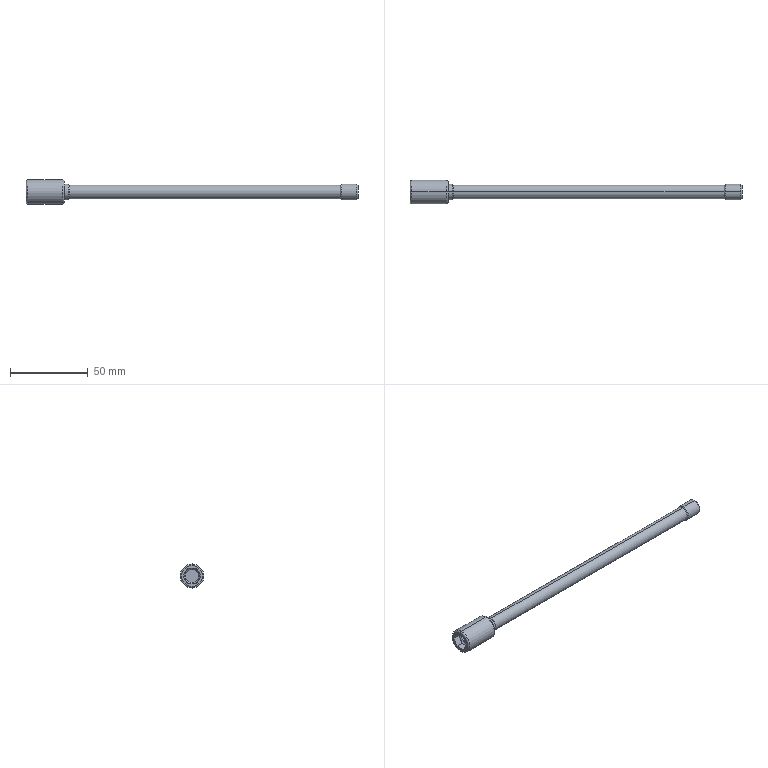Part | STEP file | SCT80_1253 | 1 solid | 38 faces | box 214 x 15.5 x 15.5 mm | volume 15558 mm3 | plane 16 | cylinder 10 | cone 8 | torus 4 | commonest cylinder face diameters 10 x4 8.376 x2 8.9 x2 15.5 x2